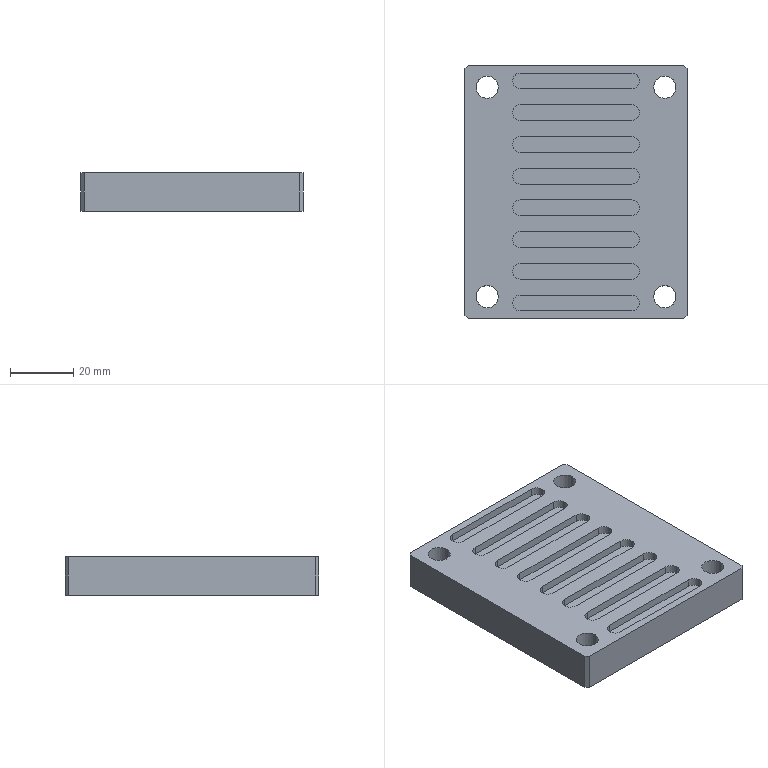Part | SolidWorks | features Chamfer 1, Extrusion 1, HoleWzd 1, ICE 1, LPattern 1 | 1 solid | 66 faces | box 70 x 80 x 12 mm | volume 61436 mm3 | plane 34 | cylinder 32 | commonest cylinder face diameters 5 x24 7 x8